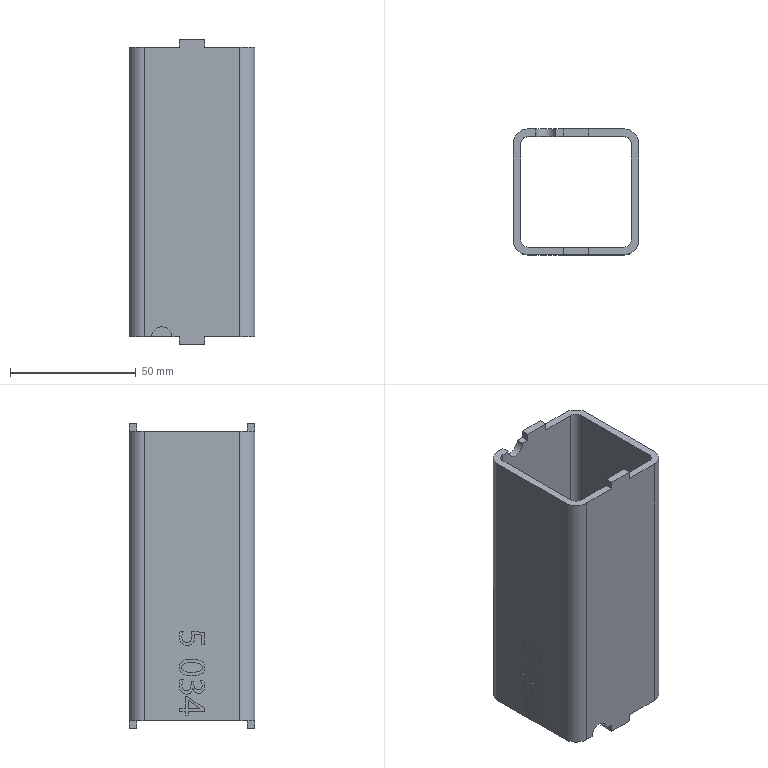Part | SolidWorks | features BaseBody 1 | 1 solid | 96 faces | box 50 x 50 x 121 mm | volume 62383 mm3 | plane 57 | spline 29 | cylinder 10 | commonest cylinder face diameters 6 x4 12 x4 8 x2